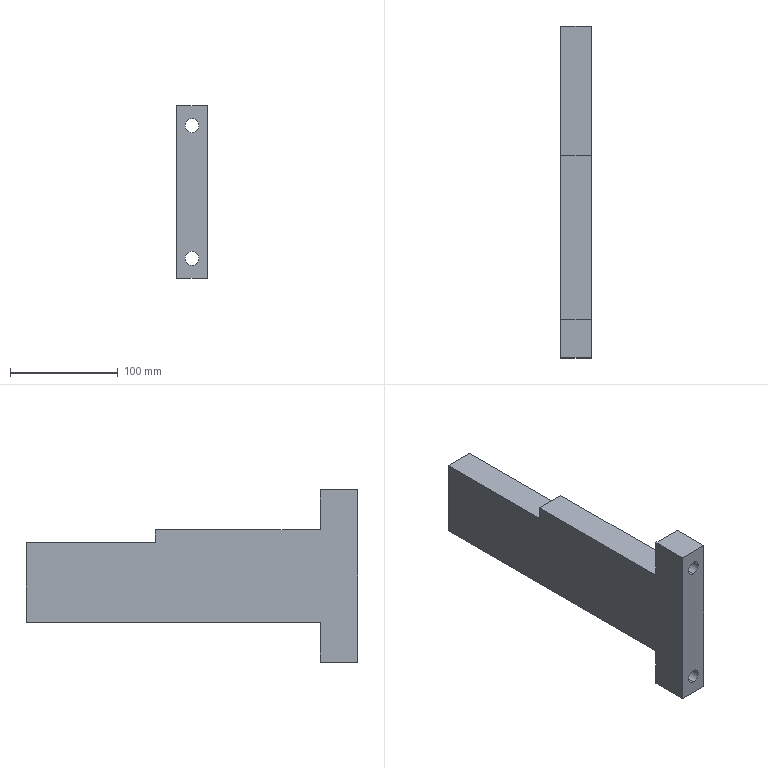Part | STEP file | PN_0014 spacer block | 1 solid | 44 faces | box 28 x 308 x 160 mm | volume 760293 mm3 | cylinder 18 | cone 14 | plane 12 | commonest cylinder face diameters 6.8 x10 5 x4 13 x4